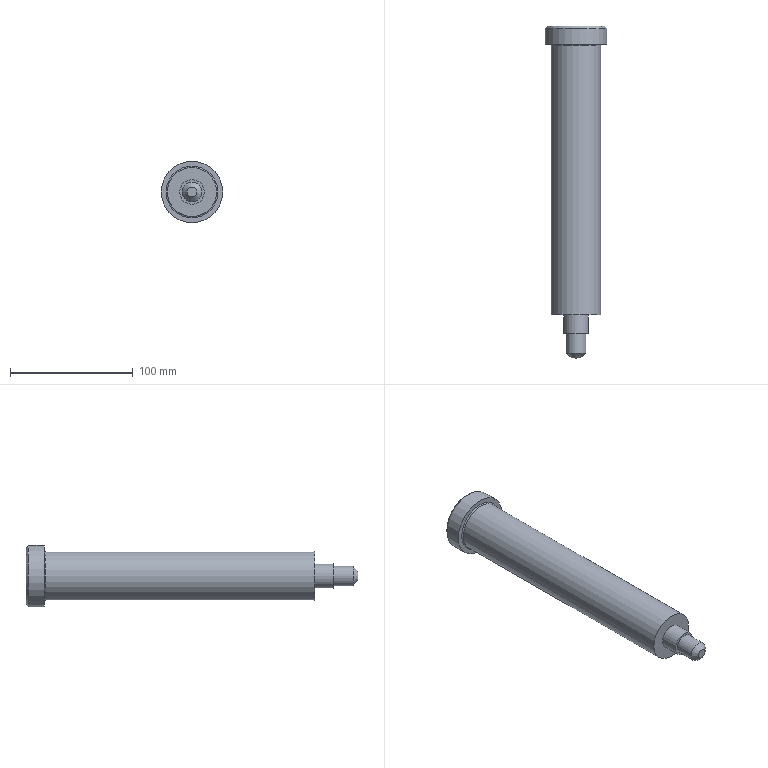Part | NX | features solid 2 | 1 solid | 12 faces | box 50 x 270 x 50 mm | volume 314033 mm3 | plane 5 | cylinder 4 | cone 2 | torus 1 | commonest cylinder face diameters 16 x1 20 x1 40 x1 50 x1
STEP:
#1=CARTESIAN_POINT('',(762.,600.,145.));
#2=VERTEX_POINT('',#1);
#3=CARTESIAN_POINT('',(785.,600.,145.));
#4=DIRECTION('',(0.,-1.,0.));
#5=DIRECTION('',(-1.,0.,0.));
#6=AXIS2_PLACEMENT_3D('',#3,#4,#5);
#7=CIRCLE('',#6,23.);
#8=EDGE_CURVE('',#2,#2,#7,.T.);
#9=ORIENTED_EDGE('',*,*,#8,.F.);
#10=EDGE_LOOP('',(#9));
#11=FACE_BOUND('',#10,.T.);
#12=CARTESIAN_POINT('',(785.,600.,145.));
#13=DIRECTION('',(0.,1.,0.));
#14=DIRECTION('',(-1.,0.,0.));
#15=AXIS2_PLACEMENT_3D('',#12,#13,#14);
#16=PLANE('',#15);
#17=ADVANCED_FACE('',(#11),#16,.T.);
#18=CARTESIAN_POINT('',(760.,598.,145.));
#19=VERTEX_POINT('',#18);
#20=CARTESIAN_POINT('',(785.,598.,145.));
#21=DIRECTION('',(0.,-1.,0.));
#22=DIRECTION('',(-1.,0.,0.));
#23=AXIS2_PLACEMENT_3D('',#20,#21,#22);
#24=CIRCLE('',#23,25.);
#25=EDGE_CURVE('',#19,#19,#24,.T.);
#26=ORIENTED_EDGE('',*,*,#25,.F.);
#27=EDGE_LOOP('',(#26));
#28=FACE_BOUND('',#27,.T.);
#29=ORIENTED_EDGE('',*,*,#8,.T.);
#30=EDGE_LOOP('',(#29));
#31=FACE_BOUND('',#30,.T.);
#32=CARTESIAN_POINT('',(785.,600.,145.));
#33=DIRECTION('',(0.,-1.,0.));
#34=DIRECTION('',(1.,0.,0.));
#35=AXIS2_PLACEMENT_3D('',#32,#33,#34);
#36=CONICAL_SURFACE('',#35,23.,0.7854);
#37=ADVANCED_FACE('',(#28,#31),#36,.T.);
#38=CARTESIAN_POINT('',(760.,585.,145.));
#39=VERTEX_POINT('',#38);
#40=CARTESIAN_POINT('',(785.,585.,145.));
#41=DIRECTION('',(0.,-1.,0.));
#42=DIRECTION('',(-1.,0.,0.));
#43=AXIS2_PLACEMENT_3D('',#40,#41,#42);
#44=CIRCLE('',#43,25.);
#45=EDGE_CURVE('',#39,#39,#44,.T.);
#46=ORIENTED_EDGE('',*,*,#45,.F.);
#47=EDGE_LOOP('',(#46));
#48=FACE_BOUND('',#47,.T.);
#49=ORIENTED_EDGE('',*,*,#25,.T.);
#50=EDGE_LOOP('',(#49));
#51=FACE_BOUND('',#50,.T.);
#52=CARTESIAN_POINT('',(785.,610.236,145.));
#53=DIRECTION('',(0.,1.,0.));
#54=DIRECTION('',(-1.,0.,0.));
#55=AXIS2_PLACEMENT_3D('',#52,#53,#54);
#56=CYLINDRICAL_SURFACE('',#55,25.);
#57=ADVANCED_FACE('',(#48,#51),#56,.T.);
#58=CARTESIAN_POINT('',(765.,584.,145.));
#59=VERTEX_POINT('',#58);
#60=CARTESIAN_POINT('',(785.,584.,145.));
#61=DIRECTION('',(0.,-1.,0.));
#62=DIRECTION('',(-1.,0.,0.));
#63=AXIS2_PLACEMENT_3D('',#60,#61,#62);
#64=CIRCLE('',#63,20.);
#65=EDGE_CURVE('',#59,#59,#64,.T.);
#66=ORIENTED_EDGE('',*,*,#65,.F.);
#67=EDGE_LOOP('',(#66));
#68=FACE_BOUND('',#67,.T.);
#69=CARTESIAN_POINT('',(764.,585.,145.));
#70=VERTEX_POINT('',#69);
#71=CARTESIAN_POINT('',(785.,585.,145.));
#72=DIRECTION('',(0.,-1.,0.));
#73=DIRECTION('',(-1.,0.,0.));
#74=AXIS2_PLACEMENT_3D('',#71,#72,#73);
#75=CIRCLE('',#74,21.);
#76=EDGE_CURVE('',#70,#70,#75,.T.);
#77=ORIENTED_EDGE('',*,*,#76,.T.);
#78=EDGE_LOOP('',(#77));
#79=FACE_BOUND('',#78,.T.);
#80=CARTESIAN_POINT('',(785.,584.,145.));
#81=DIRECTION('',(0.,1.,0.));
#82=DIRECTION('',(-1.,0.,0.));
#83=AXIS2_PLACEMENT_3D('',#80,#81,#82);
#84=TOROIDAL_SURFACE('',#83,21.,1.);
#85=ADVANCED_FACE('',(#68,#79),#84,.F.);
#86=CARTESIAN_POINT('',(765.,365.,145.));
#87=VERTEX_POINT('',#86);
#88=CARTESIAN_POINT('',(785.,365.,145.));
#89=DIRECTION('',(0.,-1.,0.));
#90=DIRECTION('',(-1.,0.,0.));
#91=AXIS2_PLACEMENT_3D('',#88,#89,#90);
#92=CIRCLE('',#91,20.);
#93=EDGE_CURVE('',#87,#87,#92,.T.);
#94=ORIENTED_EDGE('',*,*,#93,.F.);
#95=EDGE_LOOP('',(#94));
#96=FACE_BOUND('',#95,.T.);
#97=ORIENTED_EDGE('',*,*,#65,.T.);
#98=EDGE_LOOP('',(#97));
#99=FACE_BOUND('',#98,.T.);
#100=CARTESIAN_POINT('',(785.,610.236,145.));
#101=DIRECTION('',(0.,1.,0.));
#102=DIRECTION('',(-1.,0.,0.));
#103=AXIS2_PLACEMENT_3D('',#100,#101,#102);
#104=CYLINDRICAL_SURFACE('',#103,20.);
#105=ADVANCED_FACE('',(#96,#99),#104,.T.);
#106=CARTESIAN_POINT('',(775.,350.,145.));
#107=VERTEX_POINT('',#106);
#108=CARTESIAN_POINT('',(785.,350.,145.));
#109=DIRECTION('',(0.,-1.,0.));
#110=DIRECTION('',(-1.,0.,0.));
#111=AXIS2_PLACEMENT_3D('',#108,#109,#110);
#112=CIRCLE('',#111,10.);
#113=EDGE_CURVE('',#107,#107,#112,.T.);
#114=ORIENTED_EDGE('',*,*,#113,.F.);
#115=EDGE_LOOP('',(#114));
#116=FACE_BOUND('',#115,.T.);
#117=CARTESIAN_POINT('',(775.,365.,145.));
#118=VERTEX_POINT('',#117);
#119=CARTESIAN_POINT('',(785.,365.,145.));
#120=DIRECTION('',(0.,-1.,0.));
#121=DIRECTION('',(-1.,0.,0.));
#122=AXIS2_PLACEMENT_3D('',#119,#120,#121);
#123=CIRCLE('',#122,10.);
#124=EDGE_CURVE('',#118,#118,#123,.T.);
#125=ORIENTED_EDGE('',*,*,#124,.T.);
#126=EDGE_LOOP('',(#125));
#127=FACE_BOUND('',#126,.T.);
#128=CARTESIAN_POINT('',(785.,610.236,145.));
#129=DIRECTION('',(0.,1.,0.));
#130=DIRECTION('',(-1.,0.,0.));
#131=AXIS2_PLACEMENT_3D('',#128,#129,#130);
#132=CYLINDRICAL_SURFACE('',#131,10.);
#133=ADVANCED_FACE('',(#116,#127),#132,.T.);
#134=CARTESIAN_POINT('',(777.,350.,145.));
#135=VERTEX_POINT('',#134);
#136=CARTESIAN_POINT('',(785.,350.,145.));
#137=DIRECTION('',(0.,-1.,0.));
#138=DIRECTION('',(-1.,0.,0.));
#139=AXIS2_PLACEMENT_3D('',#136,#137,#138);
#140=CIRCLE('',#139,8.);
#141=EDGE_CURVE('',#135,#135,#140,.T.);
#142=ORIENTED_EDGE('',*,*,#141,.F.);
#143=EDGE_LOOP('',(#142));
#144=FACE_BOUND('',#143,.T.);
#145=ORIENTED_EDGE('',*,*,#113,.T.);
#146=EDGE_LOOP('',(#145));
#147=FACE_BOUND('',#146,.T.);
#148=CARTESIAN_POINT('',(785.,350.,135.));
#149=DIRECTION('',(0.,-1.,0.));
#150=DIRECTION('',(1.,0.,0.));
#151=AXIS2_PLACEMENT_3D('',#148,#149,#150);
#152=PLANE('',#151);
#153=ADVANCED_FACE('',(#144,#147),#152,.T.);
#154=CARTESIAN_POINT('',(777.,334.,145.));
#155=VERTEX_POINT('',#154);
#156=CARTESIAN_POINT('',(785.,334.,145.));
#157=DIRECTION('',(0.,-1.,0.));
#158=DIRECTION('',(-1.,0.,0.));
#159=AXIS2_PLACEMENT_3D('',#156,#157,#158);
#160=CIRCLE('',#159,8.);
#161=EDGE_CURVE('',#155,#155,#160,.T.);
#162=ORIENTED_EDGE('',*,*,#161,.F.);
#163=EDGE_LOOP('',(#162));
#164=FACE_BOUND('',#163,.T.);
#165=ORIENTED_EDGE('',*,*,#141,.T.);
#166=EDGE_LOOP('',(#165));
#167=FACE_BOUND('',#166,.T.);
#168=CARTESIAN_POINT('',(785.,610.236,145.));
#169=DIRECTION('',(0.,1.,0.));
#170=DIRECTION('',(-1.,0.,0.));
#171=AXIS2_PLACEMENT_3D('',#168,#169,#170);
#172=CYLINDRICAL_SURFACE('',#171,8.);
#173=ADVANCED_FACE('',(#164,#167),#172,.T.);
#174=CARTESIAN_POINT('',(781.,330.,145.));
#175=VERTEX_POINT('',#174);
#176=CARTESIAN_POINT('',(785.,330.,145.));
#177=DIRECTION('',(0.,-1.,0.));
#178=DIRECTION('',(-1.,0.,0.));
#179=AXIS2_PLACEMENT_3D('',#176,#177,#178);
#180=CIRCLE('',#179,4.);
#181=EDGE_CURVE('',#175,#175,#180,.T.);
#182=ORIENTED_EDGE('',*,*,#181,.F.);
#183=EDGE_LOOP('',(#182));
#184=FACE_BOUND('',#183,.T.);
#185=ORIENTED_EDGE('',*,*,#161,.T.);
#186=EDGE_LOOP('',(#185));
#187=FACE_BOUND('',#186,.T.);
#188=CARTESIAN_POINT('',(785.,334.,145.));
#189=DIRECTION('',(0.,1.,0.));
#190=DIRECTION('',(-1.,0.,0.));
#191=AXIS2_PLACEMENT_3D('',#188,#189,#190);
#192=CONICAL_SURFACE('',#191,8.,0.7854);
#193=ADVANCED_FACE('',(#184,#187),#192,.T.);
#194=ORIENTED_EDGE('',*,*,#181,.T.);
#195=EDGE_LOOP('',(#194));
#196=FACE_BOUND('',#195,.T.);
#197=CARTESIAN_POINT('',(785.,330.,141.));
#198=DIRECTION('',(0.,-1.,0.));
#199=DIRECTION('',(1.,0.,0.));
#200=AXIS2_PLACEMENT_3D('',#197,#198,#199);
#201=PLANE('',#200);
#202=ADVANCED_FACE('',(#196),#201,.T.);
#203=ORIENTED_EDGE('',*,*,#45,.T.);
#204=EDGE_LOOP('',(#203));
#205=FACE_BOUND('',#204,.T.);
#206=ORIENTED_EDGE('',*,*,#76,.F.);
#207=EDGE_LOOP('',(#206));
#208=FACE_BOUND('',#207,.T.);
#209=CARTESIAN_POINT('',(785.,585.,124.));
#210=DIRECTION('',(0.,1.,0.));
#211=DIRECTION('',(-1.,0.,0.));
#212=AXIS2_PLACEMENT_3D('',#209,#210,#211);
#213=PLANE('',#212);
#214=ADVANCED_FACE('',(#205,#208),#213,.F.);
#215=ORIENTED_EDGE('',*,*,#93,.T.);
#216=EDGE_LOOP('',(#215));
#217=FACE_BOUND('',#216,.T.);
#218=ORIENTED_EDGE('',*,*,#124,.F.);
#219=EDGE_LOOP('',(#218));
#220=FACE_BOUND('',#219,.T.);
#221=CARTESIAN_POINT('',(785.,365.,135.));
#222=DIRECTION('',(0.,1.,0.));
#223=DIRECTION('',(-1.,0.,0.));
#224=AXIS2_PLACEMENT_3D('',#221,#222,#223);
#225=PLANE('',#224);
#226=ADVANCED_FACE('',(#217,#220),#225,.F.);
#227=CLOSED_SHELL('',(#17,#37,#57,#85,#105,#133,#153,#173,#193,#202,#214,#226));
#228=MANIFOLD_SOLID_BREP('',#227);
#229=(LENGTH_UNIT()NAMED_UNIT(*)SI_UNIT(.MILLI.,.METRE.));
#230=UNCERTAINTY_MEASURE_WITH_UNIT(LENGTH_MEASURE(0.00001),#229,'','');
#231=(NAMED_UNIT(*)PLANE_ANGLE_UNIT()SI_UNIT($,.RADIAN.));
#232=(NAMED_UNIT(*)SI_UNIT($,.STERADIAN.)SOLID_ANGLE_UNIT());
#233=(GEOMETRIC_REPRESENTATION_CONTEXT(3)GLOBAL_UNCERTAINTY_ASSIGNED_CONTEXT((#230))GLOBAL_UNIT_ASSIGNED_CONTEXT((#229,#231,#232))REPRESENTATION_CONTEXT('',''));
#234=ADVANCED_BREP_SHAPE_REPRESENTATION('',(#228),#233);